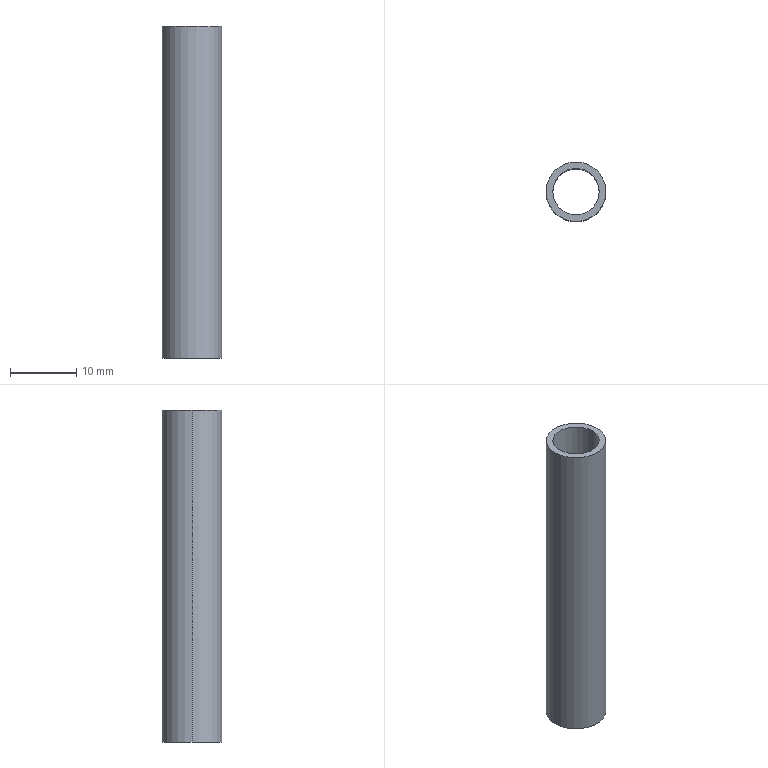Part | 1 solid | 6 faces | box 9 x 9 x 50 mm | volume 1257 mm3 | cylinder 4 | plane 2 | commonest cylinder face diameters 7 x2 9 x2
STEP:
#1=CARTESIAN_POINT('',(-3.5,0.,50.));
#2=VERTEX_POINT('',#1);
#3=CARTESIAN_POINT('',(3.5,0.,50.));
#4=VERTEX_POINT('',#3);
#5=CARTESIAN_POINT('',(0.,0.,50.));
#6=DIRECTION('',(0.,0.,1.));
#7=DIRECTION('',(1.,0.,0.));
#8=AXIS2_PLACEMENT_3D('',#5,#6,#7);
#9=CIRCLE('',#8,3.5);
#10=EDGE_CURVE('',#2,#4,#9,.T.);
#11=ORIENTED_EDGE('',*,*,#10,.T.);
#12=CARTESIAN_POINT('',(3.5,0.,0.));
#13=VERTEX_POINT('',#12);
#14=CARTESIAN_POINT('',(3.5,0.,50.));
#15=DIRECTION('',(0.,0.,-1.));
#16=VECTOR('',#15,1000.);
#17=LINE('',#14,#16);
#18=EDGE_CURVE('',#4,#13,#17,.T.);
#19=ORIENTED_EDGE('',*,*,#18,.T.);
#20=CARTESIAN_POINT('',(-3.5,0.,0.));
#21=VERTEX_POINT('',#20);
#22=CARTESIAN_POINT('',(0.,0.,0.));
#23=DIRECTION('',(0.,0.,1.));
#24=DIRECTION('',(1.,0.,0.));
#25=AXIS2_PLACEMENT_3D('',#22,#23,#24);
#26=CIRCLE('',#25,3.5);
#27=EDGE_CURVE('',#21,#13,#26,.T.);
#28=ORIENTED_EDGE('',*,*,#27,.F.);
#29=CARTESIAN_POINT('',(-3.5,0.,50.));
#30=DIRECTION('',(0.,0.,-1.));
#31=VECTOR('',#30,1000.);
#32=LINE('',#29,#31);
#33=EDGE_CURVE('',#2,#21,#32,.T.);
#34=ORIENTED_EDGE('',*,*,#33,.F.);
#35=EDGE_LOOP('',(#11,#19,#28,#34));
#36=FACE_OUTER_BOUND('',#35,.T.);
#37=CARTESIAN_POINT('',(0.,0.,50.));
#38=DIRECTION('',(0.,0.,-1.));
#39=DIRECTION('',(-1.,0.,0.));
#40=AXIS2_PLACEMENT_3D('',#37,#38,#39);
#41=CYLINDRICAL_SURFACE('',#40,3.5);
#42=ADVANCED_FACE('',(#36),#41,.F.);
#43=CARTESIAN_POINT('',(4.5,0.,50.));
#44=VERTEX_POINT('',#43);
#45=CARTESIAN_POINT('',(-4.5,0.,50.));
#46=VERTEX_POINT('',#45);
#47=CARTESIAN_POINT('',(0.,0.,50.));
#48=DIRECTION('',(0.,0.,1.));
#49=DIRECTION('',(1.,0.,0.));
#50=AXIS2_PLACEMENT_3D('',#47,#48,#49);
#51=CIRCLE('',#50,4.5);
#52=EDGE_CURVE('',#44,#46,#51,.T.);
#53=ORIENTED_EDGE('',*,*,#52,.F.);
#54=CARTESIAN_POINT('',(4.5,0.,0.));
#55=VERTEX_POINT('',#54);
#56=CARTESIAN_POINT('',(4.5,0.,50.));
#57=DIRECTION('',(0.,0.,-1.));
#58=VECTOR('',#57,1000.);
#59=LINE('',#56,#58);
#60=EDGE_CURVE('',#44,#55,#59,.T.);
#61=ORIENTED_EDGE('',*,*,#60,.T.);
#62=CARTESIAN_POINT('',(-4.5,0.,0.));
#63=VERTEX_POINT('',#62);
#64=CARTESIAN_POINT('',(0.,0.,0.));
#65=DIRECTION('',(0.,0.,1.));
#66=DIRECTION('',(1.,0.,0.));
#67=AXIS2_PLACEMENT_3D('',#64,#65,#66);
#68=CIRCLE('',#67,4.5);
#69=EDGE_CURVE('',#55,#63,#68,.T.);
#70=ORIENTED_EDGE('',*,*,#69,.T.);
#71=CARTESIAN_POINT('',(-4.5,0.,50.));
#72=DIRECTION('',(0.,0.,-1.));
#73=VECTOR('',#72,1000.);
#74=LINE('',#71,#73);
#75=EDGE_CURVE('',#46,#63,#74,.T.);
#76=ORIENTED_EDGE('',*,*,#75,.F.);
#77=EDGE_LOOP('',(#53,#61,#70,#76));
#78=FACE_OUTER_BOUND('',#77,.T.);
#79=CARTESIAN_POINT('',(0.,0.,50.));
#80=DIRECTION('',(0.,0.,-1.));
#81=DIRECTION('',(-1.,0.,0.));
#82=AXIS2_PLACEMENT_3D('',#79,#80,#81);
#83=CYLINDRICAL_SURFACE('',#82,4.5);
#84=ADVANCED_FACE('',(#78),#83,.T.);
#85=CARTESIAN_POINT('',(0.,0.,50.));
#86=DIRECTION('',(0.,0.,1.));
#87=DIRECTION('',(1.,0.,0.));
#88=AXIS2_PLACEMENT_3D('',#85,#86,#87);
#89=CIRCLE('',#88,4.5);
#90=EDGE_CURVE('',#46,#44,#89,.T.);
#91=ORIENTED_EDGE('',*,*,#90,.T.);
#92=ORIENTED_EDGE('',*,*,#52,.T.);
#93=EDGE_LOOP('',(#91,#92));
#94=FACE_OUTER_BOUND('',#93,.T.);
#95=ORIENTED_EDGE('',*,*,#10,.F.);
#96=CARTESIAN_POINT('',(0.,0.,50.));
#97=DIRECTION('',(0.,0.,1.));
#98=DIRECTION('',(1.,0.,0.));
#99=AXIS2_PLACEMENT_3D('',#96,#97,#98);
#100=CIRCLE('',#99,3.5);
#101=EDGE_CURVE('',#4,#2,#100,.T.);
#102=ORIENTED_EDGE('',*,*,#101,.F.);
#103=EDGE_LOOP('',(#95,#102));
#104=FACE_BOUND('',#103,.T.);
#105=CARTESIAN_POINT('',(0.,0.,50.));
#106=DIRECTION('',(0.,0.,1.));
#107=DIRECTION('',(1.,0.,0.));
#108=AXIS2_PLACEMENT_3D('',#105,#106,#107);
#109=PLANE('',#108);
#110=ADVANCED_FACE('',(#94,#104),#109,.T.);
#111=CARTESIAN_POINT('',(0.,0.,0.));
#112=DIRECTION('',(0.,0.,1.));
#113=DIRECTION('',(1.,0.,0.));
#114=AXIS2_PLACEMENT_3D('',#111,#112,#113);
#115=CIRCLE('',#114,4.5);
#116=EDGE_CURVE('',#63,#55,#115,.T.);
#117=ORIENTED_EDGE('',*,*,#116,.F.);
#118=ORIENTED_EDGE('',*,*,#69,.F.);
#119=EDGE_LOOP('',(#117,#118));
#120=FACE_OUTER_BOUND('',#119,.T.);
#121=ORIENTED_EDGE('',*,*,#27,.T.);
#122=CARTESIAN_POINT('',(0.,0.,0.));
#123=DIRECTION('',(0.,0.,1.));
#124=DIRECTION('',(1.,0.,0.));
#125=AXIS2_PLACEMENT_3D('',#122,#123,#124);
#126=CIRCLE('',#125,3.5);
#127=EDGE_CURVE('',#13,#21,#126,.T.);
#128=ORIENTED_EDGE('',*,*,#127,.T.);
#129=EDGE_LOOP('',(#121,#128));
#130=FACE_BOUND('',#129,.T.);
#131=CARTESIAN_POINT('',(0.,0.,0.));
#132=DIRECTION('',(0.,0.,1.));
#133=DIRECTION('',(1.,0.,0.));
#134=AXIS2_PLACEMENT_3D('',#131,#132,#133);
#135=PLANE('',#134);
#136=ADVANCED_FACE('',(#120,#130),#135,.F.);
#137=ORIENTED_EDGE('',*,*,#60,.F.);
#138=ORIENTED_EDGE('',*,*,#90,.F.);
#139=ORIENTED_EDGE('',*,*,#75,.T.);
#140=ORIENTED_EDGE('',*,*,#116,.T.);
#141=EDGE_LOOP('',(#137,#138,#139,#140));
#142=FACE_OUTER_BOUND('',#141,.T.);
#143=CARTESIAN_POINT('',(0.,0.,50.));
#144=DIRECTION('',(0.,0.,-1.));
#145=DIRECTION('',(-1.,0.,0.));
#146=AXIS2_PLACEMENT_3D('',#143,#144,#145);
#147=CYLINDRICAL_SURFACE('',#146,4.5);
#148=ADVANCED_FACE('',(#142),#147,.T.);
#149=ORIENTED_EDGE('',*,*,#18,.F.);
#150=ORIENTED_EDGE('',*,*,#101,.T.);
#151=ORIENTED_EDGE('',*,*,#33,.T.);
#152=ORIENTED_EDGE('',*,*,#127,.F.);
#153=EDGE_LOOP('',(#149,#150,#151,#152));
#154=FACE_OUTER_BOUND('',#153,.T.);
#155=CARTESIAN_POINT('',(0.,0.,50.));
#156=DIRECTION('',(0.,0.,-1.));
#157=DIRECTION('',(-1.,0.,0.));
#158=AXIS2_PLACEMENT_3D('',#155,#156,#157);
#159=CYLINDRICAL_SURFACE('',#158,3.5);
#160=ADVANCED_FACE('',(#154),#159,.F.);
#161=CLOSED_SHELL('',(#42,#84,#110,#136,#148,#160));
#162=MANIFOLD_SOLID_BREP('',#161);
#163=CARTESIAN_POINT('',(0.,0.,0.));
#164=DIRECTION('',(0.,0.,1.));
#165=DIRECTION('',(1.,0.,0.));
#166=AXIS2_PLACEMENT_3D('',#163,#164,#165);
#167=(LENGTH_UNIT()NAMED_UNIT(*)SI_UNIT(.MILLI.,.METRE.));
#168=UNCERTAINTY_MEASURE_WITH_UNIT(LENGTH_MEASURE(0.00001),#167,'','');
#169=(NAMED_UNIT(*)PLANE_ANGLE_UNIT()SI_UNIT($,.RADIAN.));
#170=(NAMED_UNIT(*)SI_UNIT($,.STERADIAN.)SOLID_ANGLE_UNIT());
#171=(GEOMETRIC_REPRESENTATION_CONTEXT(3)GLOBAL_UNCERTAINTY_ASSIGNED_CONTEXT((#168))GLOBAL_UNIT_ASSIGNED_CONTEXT((#167,#169,#170))REPRESENTATION_CONTEXT('',''));
#172=ADVANCED_BREP_SHAPE_REPRESENTATION('',(#162,#166),#171);